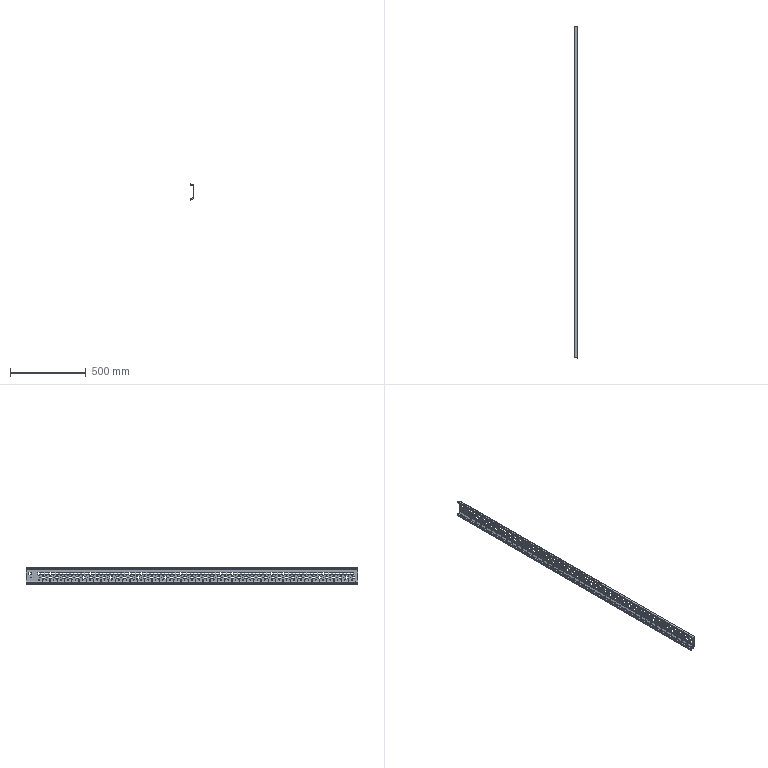Part | NX | features solid 2 | 1 solid | 1692 faces | box 26.18 x 2189 x 114 mm | volume 745580 mm3 | cylinder 1104 | plane 588 | commonest cylinder face diameters 2 x536 4.5 x532 3.2 x28 1.5 x3 6.5 x3 5 x2